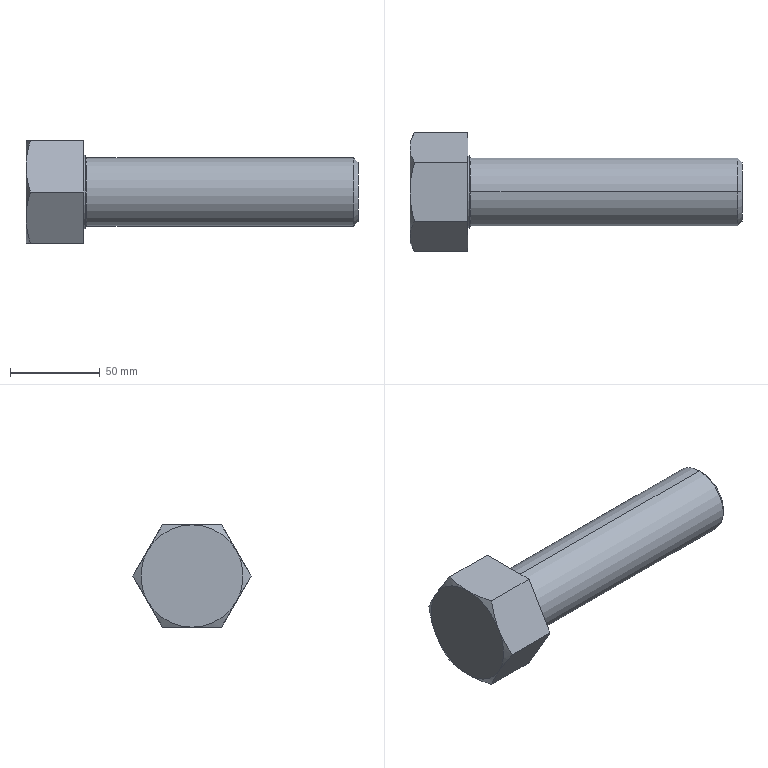Part | SolidWorks | features RevCut 4, Chamfer 1, Extrusion 1, Fillet 1, LPattern 1, Revolution 1 | 1 solid | 24 faces | box 185.42 x 65.991 x 57.15 mm | volume 265435 mm3 | plane 10 | cone 8 | cylinder 4 | torus 2 | commonest cylinder face diameters 38.1 x2 41 x2
STEP:
#1=CARTESIAN_POINT('',(34.02,0.,19.05));
#2=VERTEX_POINT('',#1);
#3=CARTESIAN_POINT('',(34.02,0.,-19.05));
#4=VERTEX_POINT('',#3);
#5=CARTESIAN_POINT('',(34.02,0.,0.));
#6=DIRECTION('',(1.,0.,0.));
#7=DIRECTION('',(0.,0.,-1.));
#8=AXIS2_PLACEMENT_3D('',#5,#6,#7);
#9=CIRCLE('',#8,19.05);
#10=EDGE_CURVE('',#2,#4,#9,.T.);
#11=ORIENTED_EDGE('',*,*,#10,.F.);
#12=CARTESIAN_POINT('',(33.02,0.,20.05));
#13=VERTEX_POINT('',#12);
#14=CARTESIAN_POINT('',(34.02,0.,20.05));
#15=DIRECTION('',(0.,1.,0.));
#16=DIRECTION('',(0.,0.,1.));
#17=AXIS2_PLACEMENT_3D('',#14,#15,#16);
#18=CIRCLE('',#17,1.);
#19=EDGE_CURVE('',#2,#13,#18,.T.);
#20=ORIENTED_EDGE('',*,*,#19,.T.);
#21=CARTESIAN_POINT('',(33.02,0.,-20.05));
#22=VERTEX_POINT('',#21);
#23=CARTESIAN_POINT('',(33.02,0.,0.));
#24=DIRECTION('',(-1.,0.,0.));
#25=DIRECTION('',(0.,0.,-1.));
#26=AXIS2_PLACEMENT_3D('',#23,#24,#25);
#27=CIRCLE('',#26,20.05);
#28=EDGE_CURVE('',#22,#13,#27,.T.);
#29=ORIENTED_EDGE('',*,*,#28,.F.);
#30=CARTESIAN_POINT('',(34.02,0.,-20.05));
#31=DIRECTION('',(0.,-1.,0.));
#32=DIRECTION('',(0.,0.,-1.));
#33=AXIS2_PLACEMENT_3D('',#30,#31,#32);
#34=CIRCLE('',#33,1.);
#35=EDGE_CURVE('',#4,#22,#34,.T.);
#36=ORIENTED_EDGE('',*,*,#35,.F.);
#37=EDGE_LOOP('',(#11,#20,#29,#36));
#38=FACE_OUTER_BOUND('',#37,.T.);
#39=CARTESIAN_POINT('',(34.02,0.,0.));
#40=DIRECTION('',(1.,0.,0.));
#41=DIRECTION('',(0.,0.,-1.));
#42=AXIS2_PLACEMENT_3D('',#39,#40,#41);
#43=TOROIDAL_SURFACE('',#42,20.05,1.);
#44=ADVANCED_FACE('',(#38),#43,.F.);
#45=CARTESIAN_POINT('',(185.42,0.,-16.65));
#46=VERTEX_POINT('',#45);
#47=CARTESIAN_POINT('',(185.42,0.,16.65));
#48=VERTEX_POINT('',#47);
#49=CARTESIAN_POINT('',(185.42,0.,0.));
#50=DIRECTION('',(1.,0.,0.));
#51=DIRECTION('',(0.,0.,1.));
#52=AXIS2_PLACEMENT_3D('',#49,#50,#51);
#53=CIRCLE('',#52,16.65);
#54=EDGE_CURVE('',#46,#48,#53,.T.);
#55=ORIENTED_EDGE('',*,*,#54,.F.);
#56=CARTESIAN_POINT('',(183.02,0.,-19.05));
#57=VERTEX_POINT('',#56);
#58=CARTESIAN_POINT('',(183.02,0.,-19.05));
#59=DIRECTION('',(-0.7071,0.,-0.7071));
#60=VECTOR('',#59,1000.);
#61=LINE('',#58,#60);
#62=EDGE_CURVE('',#46,#57,#61,.T.);
#63=ORIENTED_EDGE('',*,*,#62,.T.);
#64=CARTESIAN_POINT('',(183.02,0.,19.05));
#65=VERTEX_POINT('',#64);
#66=CARTESIAN_POINT('',(183.02,0.,0.));
#67=DIRECTION('',(-1.,0.,0.));
#68=DIRECTION('',(0.,0.,1.));
#69=AXIS2_PLACEMENT_3D('',#66,#67,#68);
#70=CIRCLE('',#69,19.05);
#71=EDGE_CURVE('',#65,#57,#70,.T.);
#72=ORIENTED_EDGE('',*,*,#71,.F.);
#73=CARTESIAN_POINT('',(183.02,0.,19.05));
#74=DIRECTION('',(-0.7071,0.,0.7071));
#75=VECTOR('',#74,1000.);
#76=LINE('',#73,#75);
#77=EDGE_CURVE('',#48,#65,#76,.T.);
#78=ORIENTED_EDGE('',*,*,#77,.F.);
#79=EDGE_LOOP('',(#55,#63,#72,#78));
#80=FACE_OUTER_BOUND('',#79,.T.);
#81=CARTESIAN_POINT('',(183.02,0.,0.));
#82=DIRECTION('',(-1.,0.,0.));
#83=DIRECTION('',(0.,0.,1.));
#84=AXIS2_PLACEMENT_3D('',#81,#82,#83);
#85=CONICAL_SURFACE('',#84,19.05,0.7854);
#86=ADVANCED_FACE('',(#80),#85,.T.);
#87=ORIENTED_EDGE('',*,*,#71,.T.);
#88=CARTESIAN_POINT('',(0.,0.,-19.05));
#89=DIRECTION('',(-1.,0.,0.));
#90=VECTOR('',#89,1000.);
#91=LINE('',#88,#90);
#92=EDGE_CURVE('',#57,#4,#91,.T.);
#93=ORIENTED_EDGE('',*,*,#92,.T.);
#94=CARTESIAN_POINT('',(34.02,0.,0.));
#95=DIRECTION('',(1.,0.,0.));
#96=DIRECTION('',(0.,0.,-1.));
#97=AXIS2_PLACEMENT_3D('',#94,#95,#96);
#98=CIRCLE('',#97,19.05);
#99=EDGE_CURVE('',#4,#2,#98,.T.);
#100=ORIENTED_EDGE('',*,*,#99,.T.);
#101=CARTESIAN_POINT('',(0.,0.,19.05));
#102=DIRECTION('',(-1.,0.,0.));
#103=VECTOR('',#102,1000.);
#104=LINE('',#101,#103);
#105=EDGE_CURVE('',#65,#2,#104,.T.);
#106=ORIENTED_EDGE('',*,*,#105,.F.);
#107=EDGE_LOOP('',(#87,#93,#100,#106));
#108=FACE_OUTER_BOUND('',#107,.T.);
#109=CARTESIAN_POINT('',(0.,0.,0.));
#110=DIRECTION('',(-1.,0.,0.));
#111=DIRECTION('',(0.,0.,1.));
#112=AXIS2_PLACEMENT_3D('',#109,#110,#111);
#113=CYLINDRICAL_SURFACE('',#112,19.05);
#114=ADVANCED_FACE('',(#108),#113,.T.);
#115=CARTESIAN_POINT('',(33.02,0.,20.5));
#116=VERTEX_POINT('',#115);
#117=CARTESIAN_POINT('',(33.02,0.,-20.5));
#118=VERTEX_POINT('',#117);
#119=CARTESIAN_POINT('',(33.02,0.,0.));
#120=DIRECTION('',(-1.,0.,0.));
#121=DIRECTION('',(0.,0.,1.));
#122=AXIS2_PLACEMENT_3D('',#119,#120,#121);
#123=CIRCLE('',#122,20.5);
#124=EDGE_CURVE('',#116,#118,#123,.T.);
#125=ORIENTED_EDGE('',*,*,#124,.T.);
#126=CARTESIAN_POINT('',(32.22,0.,-20.5));
#127=VERTEX_POINT('',#126);
#128=CARTESIAN_POINT('',(0.,0.,-20.5));
#129=DIRECTION('',(-1.,0.,0.));
#130=VECTOR('',#129,1000.);
#131=LINE('',#128,#130);
#132=EDGE_CURVE('',#118,#127,#131,.T.);
#133=ORIENTED_EDGE('',*,*,#132,.T.);
#134=CARTESIAN_POINT('',(32.22,0.,20.5));
#135=VERTEX_POINT('',#134);
#136=CARTESIAN_POINT('',(32.22,0.,0.));
#137=DIRECTION('',(-1.,0.,0.));
#138=DIRECTION('',(0.,0.,1.));
#139=AXIS2_PLACEMENT_3D('',#136,#137,#138);
#140=CIRCLE('',#139,20.5);
#141=EDGE_CURVE('',#135,#127,#140,.T.);
#142=ORIENTED_EDGE('',*,*,#141,.F.);
#143=CARTESIAN_POINT('',(0.,0.,20.5));
#144=DIRECTION('',(-1.,0.,0.));
#145=VECTOR('',#144,1000.);
#146=LINE('',#143,#145);
#147=EDGE_CURVE('',#116,#135,#146,.T.);
#148=ORIENTED_EDGE('',*,*,#147,.F.);
#149=EDGE_LOOP('',(#125,#133,#142,#148));
#150=FACE_OUTER_BOUND('',#149,.T.);
#151=CARTESIAN_POINT('',(0.,0.,0.));
#152=DIRECTION('',(-1.,0.,0.));
#153=DIRECTION('',(0.,0.,1.));
#154=AXIS2_PLACEMENT_3D('',#151,#152,#153);
#155=CYLINDRICAL_SURFACE('',#154,20.5);
#156=ADVANCED_FACE('',(#150),#155,.T.);
#157=CARTESIAN_POINT('',(32.22,16.498,-28.575));
#158=VERTEX_POINT('',#157);
#159=CARTESIAN_POINT('',(32.22,32.996,0.));
#160=VERTEX_POINT('',#159);
#161=CARTESIAN_POINT('',(32.22,16.498,-28.575));
#162=DIRECTION('',(0.,0.5,0.866));
#163=VECTOR('',#162,1000.);
#164=LINE('',#161,#163);
#165=EDGE_CURVE('',#158,#160,#164,.T.);
#166=ORIENTED_EDGE('',*,*,#165,.F.);
#167=CARTESIAN_POINT('',(2.552,16.498,-28.575));
#168=VERTEX_POINT('',#167);
#169=CARTESIAN_POINT('',(33.02,16.498,-28.575));
#170=DIRECTION('',(-1.,0.,0.));
#171=VECTOR('',#170,1000.);
#172=LINE('',#169,#171);
#173=EDGE_CURVE('',#158,#168,#172,.T.);
#174=ORIENTED_EDGE('',*,*,#173,.T.);
#175=CARTESIAN_POINT('',(0.,24.747,-14.288));
#176=VERTEX_POINT('',#175);
#177=CARTESIAN_POINT('',(0.,24.747,-14.288));
#178=CARTESIAN_POINT('',(0.,24.397,-14.894));
#179=CARTESIAN_POINT('',(0.01497,24.045,-15.503));
#180=CARTESIAN_POINT('',(0.07434,23.345,-16.716));
#181=CARTESIAN_POINT('',(0.1187,22.996,-17.32));
#182=CARTESIAN_POINT('',(0.2938,21.952,-19.127));
#183=CARTESIAN_POINT('',(0.4667,21.261,-20.324));
#184=CARTESIAN_POINT('',(1.134,19.201,-23.893));
#185=CARTESIAN_POINT('',(1.775,17.844,-26.244));
#186=CARTESIAN_POINT('',(2.552,16.498,-28.575));
#187=B_SPLINE_CURVE_WITH_KNOTS('',3,(#177,#178,#179,#180,#181,#182,#183,#184,#185,#186),.UNSPECIFIED.,.F.,.F.,(4,2,2,2,4),(0.01669,0.01877,0.02085,0.02501,0.03332),.UNSPECIFIED.);
#188=EDGE_CURVE('',#176,#168,#187,.T.);
#189=ORIENTED_EDGE('',*,*,#188,.F.);
#190=CARTESIAN_POINT('',(2.552,32.996,0.));
#191=VERTEX_POINT('',#190);
#192=CARTESIAN_POINT('',(2.552,32.996,0.));
#193=CARTESIAN_POINT('',(1.773,31.646,-2.337));
#194=CARTESIAN_POINT('',(1.131,30.287,-4.692));
#195=CARTESIAN_POINT('',(0.2432,27.54,-9.449));
#196=CARTESIAN_POINT('',(0.,26.152,-11.853));
#197=CARTESIAN_POINT('',(0.,24.747,-14.288));
#198=B_SPLINE_CURVE_WITH_KNOTS('',3,(#192,#193,#194,#195,#196,#197),.UNSPECIFIED.,.F.,.F.,(4,2,4),(0.000000238,0.008347,0.01669),.UNSPECIFIED.);
#199=EDGE_CURVE('',#191,#176,#198,.T.);
#200=ORIENTED_EDGE('',*,*,#199,.F.);
#201=CARTESIAN_POINT('',(33.02,32.996,0.));
#202=DIRECTION('',(-1.,0.,0.));
#203=VECTOR('',#202,1000.);
#204=LINE('',#201,#203);
#205=EDGE_CURVE('',#160,#191,#204,.T.);
#206=ORIENTED_EDGE('',*,*,#205,.F.);
#207=EDGE_LOOP('',(#166,#174,#189,#200,#206));
#208=FACE_OUTER_BOUND('',#207,.T.);
#209=CARTESIAN_POINT('',(33.02,16.498,-28.575));
#210=DIRECTION('',(0.,-0.866,0.5));
#211=DIRECTION('',(0.,-0.5,-0.866));
#212=AXIS2_PLACEMENT_3D('',#209,#210,#211);
#213=PLANE('',#212);
#214=ADVANCED_FACE('',(#208),#213,.F.);
#215=CARTESIAN_POINT('',(32.22,16.498,28.575));
#216=VERTEX_POINT('',#215);
#217=CARTESIAN_POINT('',(32.22,32.996,0.));
#218=DIRECTION('',(0.,-0.5,0.866));
#219=VECTOR('',#218,1000.);
#220=LINE('',#217,#219);
#221=EDGE_CURVE('',#160,#216,#220,.T.);
#222=ORIENTED_EDGE('',*,*,#221,.F.);
#223=ORIENTED_EDGE('',*,*,#205,.T.);
#224=CARTESIAN_POINT('',(0.,24.747,14.288));
#225=VERTEX_POINT('',#224);
#226=CARTESIAN_POINT('',(0.,24.747,14.288));
#227=CARTESIAN_POINT('',(0.,25.097,13.681));
#228=CARTESIAN_POINT('',(0.01497,25.448,13.072));
#229=CARTESIAN_POINT('',(0.07434,26.149,11.859));
#230=CARTESIAN_POINT('',(0.1187,26.498,11.255));
#231=CARTESIAN_POINT('',(0.2938,27.541,9.448));
#232=CARTESIAN_POINT('',(0.4667,28.232,8.251));
#233=CARTESIAN_POINT('',(1.134,30.292,4.682));
#234=CARTESIAN_POINT('',(1.775,31.65,2.331));
#235=CARTESIAN_POINT('',(2.552,32.996,0.));
#236=B_SPLINE_CURVE_WITH_KNOTS('',3,(#226,#227,#228,#229,#230,#231,#232,#233,#234,#235),.UNSPECIFIED.,.F.,.F.,(4,2,2,2,4),(0.01669,0.01877,0.02085,0.02501,0.03332),.UNSPECIFIED.);
#237=EDGE_CURVE('',#225,#191,#236,.T.);
#238=ORIENTED_EDGE('',*,*,#237,.F.);
#239=CARTESIAN_POINT('',(2.552,16.498,28.575));
#240=VERTEX_POINT('',#239);
#241=CARTESIAN_POINT('',(2.552,16.498,28.575));
#242=CARTESIAN_POINT('',(1.773,17.847,26.238));
#243=CARTESIAN_POINT('',(1.131,19.206,23.883));
#244=CARTESIAN_POINT('',(0.2432,21.953,19.126));
#245=CARTESIAN_POINT('',(0.,23.341,16.722));
#246=CARTESIAN_POINT('',(0.,24.747,14.288));
#247=B_SPLINE_CURVE_WITH_KNOTS('',3,(#241,#242,#243,#244,#245,#246),.UNSPECIFIED.,.F.,.F.,(4,2,4),(0.000000238,0.008347,0.01669),.UNSPECIFIED.);
#248=EDGE_CURVE('',#240,#225,#247,.T.);
#249=ORIENTED_EDGE('',*,*,#248,.F.);
#250=CARTESIAN_POINT('',(33.02,16.498,28.575));
#251=DIRECTION('',(-1.,0.,0.));
#252=VECTOR('',#251,1000.);
#253=LINE('',#250,#252);
#254=EDGE_CURVE('',#216,#240,#253,.T.);
#255=ORIENTED_EDGE('',*,*,#254,.F.);
#256=EDGE_LOOP('',(#222,#223,#238,#249,#255));
#257=FACE_OUTER_BOUND('',#256,.T.);
#258=CARTESIAN_POINT('',(33.02,32.996,0.));
#259=DIRECTION('',(0.,-0.866,-0.5));
#260=DIRECTION('',(0.,0.5,-0.866));
#261=AXIS2_PLACEMENT_3D('',#258,#259,#260);
#262=PLANE('',#261);
#263=ADVANCED_FACE('',(#257),#262,.F.);
#264=CARTESIAN_POINT('',(32.22,-16.498,28.575));
#265=VERTEX_POINT('',#264);
#266=CARTESIAN_POINT('',(32.22,16.498,28.575));
#267=DIRECTION('',(0.,-1.,0.));
#268=VECTOR('',#267,1000.);
#269=LINE('',#266,#268);
#270=EDGE_CURVE('',#216,#265,#269,.T.);
#271=ORIENTED_EDGE('',*,*,#270,.F.);
#272=ORIENTED_EDGE('',*,*,#254,.T.);
#273=CARTESIAN_POINT('',(0.,0.,28.575));
#274=VERTEX_POINT('',#273);
#275=CARTESIAN_POINT('',(0.,0.,28.575));
#276=CARTESIAN_POINT('',(0.,1.395,28.575));
#277=CARTESIAN_POINT('',(0.05934,2.796,28.575));
#278=CARTESIAN_POINT('',(0.2953,5.606,28.575));
#279=CARTESIAN_POINT('',(0.4701,6.996,28.575));
#280=CARTESIAN_POINT('',(1.141,11.128,28.575));
#281=CARTESIAN_POINT('',(1.782,13.83,28.575));
#282=CARTESIAN_POINT('',(2.552,16.498,28.575));
#283=B_SPLINE_CURVE_WITH_KNOTS('',3,(#275,#276,#277,#278,#279,#280,#281,#282),.UNSPECIFIED.,.F.,.F.,(4,2,2,4),(0.04657,0.05075,0.05493,0.06328),.UNSPECIFIED.);
#284=EDGE_CURVE('',#274,#240,#283,.T.);
#285=ORIENTED_EDGE('',*,*,#284,.F.);
#286=CARTESIAN_POINT('',(2.552,-16.498,28.575));
#287=VERTEX_POINT('',#286);
#288=CARTESIAN_POINT('',(2.552,-16.498,28.575));
#289=CARTESIAN_POINT('',(2.165,-15.156,28.575));
#290=CARTESIAN_POINT('',(1.809,-13.8,28.575));
#291=CARTESIAN_POINT('',(1.178,-11.061,28.575));
#292=CARTESIAN_POINT('',(0.9058,-9.689,28.575));
#293=CARTESIAN_POINT('',(0.2398,-5.559,28.575));
#294=CARTESIAN_POINT('',(0.,-2.789,28.575));
#295=CARTESIAN_POINT('',(0.,0.,28.575));
#296=B_SPLINE_CURVE_WITH_KNOTS('',3,(#288,#289,#290,#291,#292,#293,#294,#295),.UNSPECIFIED.,.F.,.F.,(4,2,2,4),(0.02988,0.03405,0.03823,0.04657),.UNSPECIFIED.);
#297=EDGE_CURVE('',#287,#274,#296,.T.);
#298=ORIENTED_EDGE('',*,*,#297,.F.);
#299=CARTESIAN_POINT('',(33.02,-16.498,28.575));
#300=DIRECTION('',(-1.,0.,0.));
#301=VECTOR('',#300,1000.);
#302=LINE('',#299,#301);
#303=EDGE_CURVE('',#265,#287,#302,.T.);
#304=ORIENTED_EDGE('',*,*,#303,.F.);
#305=EDGE_LOOP('',(#271,#272,#285,#298,#304));
#306=FACE_OUTER_BOUND('',#305,.T.);
#307=CARTESIAN_POINT('',(33.02,16.498,28.575));
#308=DIRECTION('',(0.,0.,-1.));
#309=DIRECTION('',(0.,1.,0.));
#310=AXIS2_PLACEMENT_3D('',#307,#308,#309);
#311=PLANE('',#310);
#312=ADVANCED_FACE('',(#306),#311,.F.);
#313=CARTESIAN_POINT('',(32.22,-32.996,0.));
#314=VERTEX_POINT('',#313);
#315=CARTESIAN_POINT('',(32.22,-32.996,0.));
#316=DIRECTION('',(0.,-0.5,-0.866));
#317=VECTOR('',#316,1000.);
#318=LINE('',#315,#317);
#319=EDGE_CURVE('',#265,#314,#318,.T.);
#320=ORIENTED_EDGE('',*,*,#319,.F.);
#321=ORIENTED_EDGE('',*,*,#303,.T.);
#322=CARTESIAN_POINT('',(0.,-24.747,14.288));
#323=VERTEX_POINT('',#322);
#324=CARTESIAN_POINT('',(0.,-24.747,14.288));
#325=CARTESIAN_POINT('',(0.,-24.397,14.894));
#326=CARTESIAN_POINT('',(0.01497,-24.045,15.503));
#327=CARTESIAN_POINT('',(0.07434,-23.345,16.716));
#328=CARTESIAN_POINT('',(0.1187,-22.996,17.32));
#329=CARTESIAN_POINT('',(0.2938,-21.952,19.127));
#330=CARTESIAN_POINT('',(0.4667,-21.261,20.324));
#331=CARTESIAN_POINT('',(1.134,-19.201,23.893));
#332=CARTESIAN_POINT('',(1.775,-17.844,26.244));
#333=CARTESIAN_POINT('',(2.552,-16.498,28.575));
#334=B_SPLINE_CURVE_WITH_KNOTS('',3,(#324,#325,#326,#327,#328,#329,#330,#331,#332,#333),.UNSPECIFIED.,.F.,.F.,(4,2,2,2,4),(0.01669,0.01877,0.02085,0.02501,0.03332),.UNSPECIFIED.);
#335=EDGE_CURVE('',#323,#287,#334,.T.);
#336=ORIENTED_EDGE('',*,*,#335,.F.);
#337=CARTESIAN_POINT('',(2.552,-32.996,0.));
#338=VERTEX_POINT('',#337);
#339=CARTESIAN_POINT('',(2.552,-32.996,0.));
#340=CARTESIAN_POINT('',(1.773,-31.646,2.337));
#341=CARTESIAN_POINT('',(1.131,-30.287,4.692));
#342=CARTESIAN_POINT('',(0.2432,-27.54,9.449));
#343=CARTESIAN_POINT('',(0.,-26.152,11.853));
#344=CARTESIAN_POINT('',(0.,-24.747,14.288));
#345=B_SPLINE_CURVE_WITH_KNOTS('',3,(#339,#340,#341,#342,#343,#344),.UNSPECIFIED.,.F.,.F.,(4,2,4),(0.000000238,0.008347,0.01669),.UNSPECIFIED.);
#346=EDGE_CURVE('',#338,#323,#345,.T.);
#347=ORIENTED_EDGE('',*,*,#346,.F.);
#348=CARTESIAN_POINT('',(33.02,-32.996,0.));
#349=DIRECTION('',(-1.,0.,0.));
#350=VECTOR('',#349,1000.);
#351=LINE('',#348,#350);
#352=EDGE_CURVE('',#314,#338,#351,.T.);
#353=ORIENTED_EDGE('',*,*,#352,.F.);
#354=EDGE_LOOP('',(#320,#321,#336,#347,#353));
#355=FACE_OUTER_BOUND('',#354,.T.);
#356=CARTESIAN_POINT('',(33.02,-32.996,0.));
#357=DIRECTION('',(0.,0.866,-0.5));
#358=DIRECTION('',(0.,0.5,0.866));
#359=AXIS2_PLACEMENT_3D('',#356,#357,#358);
#360=PLANE('',#359);
#361=ADVANCED_FACE('',(#355),#360,.F.);
#362=CARTESIAN_POINT('',(32.22,-16.498,-28.575));
#363=VERTEX_POINT('',#362);
#364=CARTESIAN_POINT('',(32.22,-16.498,-28.575));
#365=DIRECTION('',(0.,0.5,-0.866));
#366=VECTOR('',#365,1000.);
#367=LINE('',#364,#366);
#368=EDGE_CURVE('',#314,#363,#367,.T.);
#369=ORIENTED_EDGE('',*,*,#368,.F.);
#370=ORIENTED_EDGE('',*,*,#352,.T.);
#371=CARTESIAN_POINT('',(0.,-24.747,-14.288));
#372=VERTEX_POINT('',#371);
#373=CARTESIAN_POINT('',(0.,-24.747,-14.288));
#374=CARTESIAN_POINT('',(0.,-25.097,-13.681));
#375=CARTESIAN_POINT('',(0.01497,-25.448,-13.072));
#376=CARTESIAN_POINT('',(0.07434,-26.149,-11.859));
#377=CARTESIAN_POINT('',(0.1187,-26.498,-11.255));
#378=CARTESIAN_POINT('',(0.2938,-27.541,-9.448));
#379=CARTESIAN_POINT('',(0.4667,-28.232,-8.251));
#380=CARTESIAN_POINT('',(1.134,-30.292,-4.682));
#381=CARTESIAN_POINT('',(1.775,-31.65,-2.331));
#382=CARTESIAN_POINT('',(2.552,-32.996,0.));
#383=B_SPLINE_CURVE_WITH_KNOTS('',3,(#373,#374,#375,#376,#377,#378,#379,#380,#381,#382),.UNSPECIFIED.,.F.,.F.,(4,2,2,2,4),(0.01669,0.01877,0.02085,0.02501,0.03332),.UNSPECIFIED.);
#384=EDGE_CURVE('',#372,#338,#383,.T.);
#385=ORIENTED_EDGE('',*,*,#384,.F.);
#386=CARTESIAN_POINT('',(2.552,-16.498,-28.575));
#387=VERTEX_POINT('',#386);
#388=CARTESIAN_POINT('',(2.552,-16.498,-28.575));
#389=CARTESIAN_POINT('',(1.773,-17.847,-26.238));
#390=CARTESIAN_POINT('',(1.131,-19.206,-23.883));
#391=CARTESIAN_POINT('',(0.2432,-21.953,-19.126));
#392=CARTESIAN_POINT('',(0.,-23.341,-16.722));
#393=CARTESIAN_POINT('',(0.,-24.747,-14.288));
#394=B_SPLINE_CURVE_WITH_KNOTS('',3,(#388,#389,#390,#391,#392,#393),.UNSPECIFIED.,.F.,.F.,(4,2,4),(0.000000238,0.008347,0.01669),.UNSPECIFIED.);
#395=EDGE_CURVE('',#387,#372,#394,.T.);
#396=ORIENTED_EDGE('',*,*,#395,.F.);
#397=CARTESIAN_POINT('',(33.02,-16.498,-28.575));
#398=DIRECTION('',(-1.,0.,0.));
#399=VECTOR('',#398,1000.);
#400=LINE('',#397,#399);
#401=EDGE_CURVE('',#363,#387,#400,.T.);
#402=ORIENTED_EDGE('',*,*,#401,.F.);
#403=EDGE_LOOP('',(#369,#370,#385,#396,#402));
#404=FACE_OUTER_BOUND('',#403,.T.);
#405=CARTESIAN_POINT('',(33.02,-16.498,-28.575));
#406=DIRECTION('',(0.,0.866,0.5));
#407=DIRECTION('',(0.,-0.5,0.866));
#408=AXIS2_PLACEMENT_3D('',#405,#406,#407);
#409=PLANE('',#408);
#410=ADVANCED_FACE('',(#404),#409,.F.);
#411=CARTESIAN_POINT('',(32.22,16.498,-28.575));
#412=DIRECTION('',(0.,1.,0.));
#413=VECTOR('',#412,1000.);
#414=LINE('',#411,#413);
#415=EDGE_CURVE('',#363,#158,#414,.T.);
#416=ORIENTED_EDGE('',*,*,#415,.F.);
#417=ORIENTED_EDGE('',*,*,#401,.T.);
#418=CARTESIAN_POINT('',(0.,0.,-28.575));
#419=VERTEX_POINT('',#418);
#420=CARTESIAN_POINT('',(0.,0.,-28.575));
#421=CARTESIAN_POINT('',(0.,-2.789,-28.575));
#422=CARTESIAN_POINT('',(0.2398,-5.559,-28.575));
#423=CARTESIAN_POINT('',(0.9058,-9.689,-28.575));
#424=CARTESIAN_POINT('',(1.178,-11.061,-28.575));
#425=CARTESIAN_POINT('',(1.809,-13.8,-28.575));
#426=CARTESIAN_POINT('',(2.165,-15.156,-28.575));
#427=CARTESIAN_POINT('',(2.552,-16.498,-28.575));
#428=B_SPLINE_CURVE_WITH_KNOTS('',3,(#420,#421,#422,#423,#424,#425,#426,#427),.UNSPECIFIED.,.F.,.F.,(4,2,2,4),(0.09019,0.09855,0.1027,0.1069),.UNSPECIFIED.);
#429=EDGE_CURVE('',#419,#387,#428,.T.);
#430=ORIENTED_EDGE('',*,*,#429,.F.);
#431=CARTESIAN_POINT('',(2.552,16.498,-28.575));
#432=CARTESIAN_POINT('',(1.782,13.83,-28.575));
#433=CARTESIAN_POINT('',(1.141,11.128,-28.575));
#434=CARTESIAN_POINT('',(0.4701,6.996,-28.575));
#435=CARTESIAN_POINT('',(0.2953,5.606,-28.575));
#436=CARTESIAN_POINT('',(0.05934,2.796,-28.575));
#437=CARTESIAN_POINT('',(0.,1.395,-28.575));
#438=CARTESIAN_POINT('',(0.,0.,-28.575));
#439=B_SPLINE_CURVE_WITH_KNOTS('',3,(#431,#432,#433,#434,#435,#436,#437,#438),.UNSPECIFIED.,.F.,.F.,(4,2,2,4),(0.07347,0.08183,0.08601,0.09019),.UNSPECIFIED.);
#440=EDGE_CURVE('',#168,#419,#439,.T.);
#441=ORIENTED_EDGE('',*,*,#440,.F.);
#442=ORIENTED_EDGE('',*,*,#173,.F.);
#443=EDGE_LOOP('',(#416,#417,#430,#441,#442));
#444=FACE_OUTER_BOUND('',#443,.T.);
#445=CARTESIAN_POINT('',(33.02,16.498,-28.575));
#446=DIRECTION('',(0.,0.,1.));
#447=DIRECTION('',(0.,-1.,0.));
#448=AXIS2_PLACEMENT_3D('',#445,#446,#447);
#449=PLANE('',#448);
#450=ADVANCED_FACE('',(#444),#449,.F.);
#451=ORIENTED_EDGE('',*,*,#395,.T.);
#452=CARTESIAN_POINT('',(0.,0.,0.));
#453=DIRECTION('',(1.,0.,0.));
#454=DIRECTION('',(0.,0.,-1.));
#455=AXIS2_PLACEMENT_3D('',#452,#453,#454);
#456=CIRCLE('',#455,28.575);
#457=EDGE_CURVE('',#372,#419,#456,.T.);
#458=ORIENTED_EDGE('',*,*,#457,.T.);
#459=ORIENTED_EDGE('',*,*,#429,.T.);
#460=EDGE_LOOP('',(#451,#458,#459));
#461=FACE_OUTER_BOUND('',#460,.T.);
#462=CARTESIAN_POINT('',(0.,0.,0.));
#463=DIRECTION('',(1.,0.,0.));
#464=DIRECTION('',(0.,0.,-1.));
#465=AXIS2_PLACEMENT_3D('',#462,#463,#464);
#466=CONICAL_SURFACE('',#465,28.575,1.047);
#467=ADVANCED_FACE('',(#461),#466,.T.);
#468=ORIENTED_EDGE('',*,*,#346,.T.);
#469=CARTESIAN_POINT('',(0.,0.,0.));
#470=DIRECTION('',(1.,0.,0.));
#471=DIRECTION('',(0.,0.,-1.));
#472=AXIS2_PLACEMENT_3D('',#469,#470,#471);
#473=CIRCLE('',#472,28.575);
#474=EDGE_CURVE('',#323,#372,#473,.T.);
#475=ORIENTED_EDGE('',*,*,#474,.T.);
#476=ORIENTED_EDGE('',*,*,#384,.T.);
#477=EDGE_LOOP('',(#468,#475,#476));
#478=FACE_OUTER_BOUND('',#477,.T.);
#479=CARTESIAN_POINT('',(0.,0.,0.));
#480=DIRECTION('',(1.,0.,0.));
#481=DIRECTION('',(0.,0.,-1.));
#482=AXIS2_PLACEMENT_3D('',#479,#480,#481);
#483=CONICAL_SURFACE('',#482,28.575,1.047);
#484=ADVANCED_FACE('',(#478),#483,.T.);
#485=ORIENTED_EDGE('',*,*,#297,.T.);
#486=CARTESIAN_POINT('',(0.,0.,0.));
#487=DIRECTION('',(1.,0.,0.));
#488=DIRECTION('',(0.,0.,-1.));
#489=AXIS2_PLACEMENT_3D('',#486,#487,#488);
#490=CIRCLE('',#489,28.575);
#491=EDGE_CURVE('',#274,#323,#490,.T.);
#492=ORIENTED_EDGE('',*,*,#491,.T.);
#493=ORIENTED_EDGE('',*,*,#335,.T.);
#494=EDGE_LOOP('',(#485,#492,#493));
#495=FACE_OUTER_BOUND('',#494,.T.);
#496=CARTESIAN_POINT('',(0.,0.,0.));
#497=DIRECTION('',(1.,0.,0.));
#498=DIRECTION('',(0.,0.,-1.));
#499=AXIS2_PLACEMENT_3D('',#496,#497,#498);
#500=CONICAL_SURFACE('',#499,28.575,1.047);
#501=ADVANCED_FACE('',(#495),#500,.T.);
#502=ORIENTED_EDGE('',*,*,#284,.T.);
#503=ORIENTED_EDGE('',*,*,#248,.T.);
#504=CARTESIAN_POINT('',(0.,0.,0.));
#505=DIRECTION('',(-1.,0.,0.));
#506=DIRECTION('',(0.,0.,1.));
#507=AXIS2_PLACEMENT_3D('',#504,#505,#506);
#508=CIRCLE('',#507,28.575);
#509=EDGE_CURVE('',#274,#225,#508,.T.);
#510=ORIENTED_EDGE('',*,*,#509,.F.);
#511=EDGE_LOOP('',(#502,#503,#510));
#512=FACE_OUTER_BOUND('',#511,.T.);
#513=CARTESIAN_POINT('',(0.,0.,0.));
#514=DIRECTION('',(1.,0.,0.));
#515=DIRECTION('',(0.,0.,-1.));
#516=AXIS2_PLACEMENT_3D('',#513,#514,#515);
#517=CONICAL_SURFACE('',#516,28.575,1.047);
#518=ADVANCED_FACE('',(#512),#517,.T.);
#519=ORIENTED_EDGE('',*,*,#237,.T.);
#520=ORIENTED_EDGE('',*,*,#199,.T.);
#521=CARTESIAN_POINT('',(0.,0.,0.));
#522=DIRECTION('',(1.,0.,0.));
#523=DIRECTION('',(0.,0.,-1.));
#524=AXIS2_PLACEMENT_3D('',#521,#522,#523);
#525=CIRCLE('',#524,28.575);
#526=EDGE_CURVE('',#176,#225,#525,.T.);
#527=ORIENTED_EDGE('',*,*,#526,.T.);
#528=EDGE_LOOP('',(#519,#520,#527));
#529=FACE_OUTER_BOUND('',#528,.T.);
#530=CARTESIAN_POINT('',(0.,0.,0.));
#531=DIRECTION('',(1.,0.,0.));
#532=DIRECTION('',(0.,0.,-1.));
#533=AXIS2_PLACEMENT_3D('',#530,#531,#532);
#534=CONICAL_SURFACE('',#533,28.575,1.047);
#535=ADVANCED_FACE('',(#529),#534,.T.);
#536=ORIENTED_EDGE('',*,*,#188,.T.);
#537=ORIENTED_EDGE('',*,*,#440,.T.);
#538=CARTESIAN_POINT('',(0.,0.,0.));
#539=DIRECTION('',(1.,0.,0.));
#540=DIRECTION('',(0.,0.,-1.));
#541=AXIS2_PLACEMENT_3D('',#538,#539,#540);
#542=CIRCLE('',#541,28.575);
#543=EDGE_CURVE('',#419,#176,#542,.T.);
#544=ORIENTED_EDGE('',*,*,#543,.T.);
#545=EDGE_LOOP('',(#536,#537,#544));
#546=FACE_OUTER_BOUND('',#545,.T.);
#547=CARTESIAN_POINT('',(0.,0.,0.));
#548=DIRECTION('',(1.,0.,0.));
#549=DIRECTION('',(0.,0.,-1.));
#550=AXIS2_PLACEMENT_3D('',#547,#548,#549);
#551=CONICAL_SURFACE('',#550,28.575,1.047);
#552=ADVANCED_FACE('',(#546),#551,.T.);
#553=ORIENTED_EDGE('',*,*,#543,.F.);
#554=ORIENTED_EDGE('',*,*,#457,.F.);
#555=ORIENTED_EDGE('',*,*,#474,.F.);
#556=ORIENTED_EDGE('',*,*,#491,.F.);
#557=ORIENTED_EDGE('',*,*,#509,.T.);
#558=ORIENTED_EDGE('',*,*,#526,.F.);
#559=EDGE_LOOP('',(#553,#554,#555,#556,#557,#558));
#560=FACE_OUTER_BOUND('',#559,.T.);
#561=CARTESIAN_POINT('',(0.,0.,-57.15));
#562=DIRECTION('',(1.,0.,0.));
#563=DIRECTION('',(0.,0.,-1.));
#564=AXIS2_PLACEMENT_3D('',#561,#562,#563);
#565=PLANE('',#564);
#566=ADVANCED_FACE('',(#560),#565,.F.);
#567=ORIENTED_EDGE('',*,*,#141,.T.);
#568=CARTESIAN_POINT('',(32.22,0.,0.));
#569=DIRECTION('',(-1.,0.,0.));
#570=DIRECTION('',(0.,0.,1.));
#571=AXIS2_PLACEMENT_3D('',#568,#569,#570);
#572=CIRCLE('',#571,20.5);
#573=EDGE_CURVE('',#127,#135,#572,.T.);
#574=ORIENTED_EDGE('',*,*,#573,.T.);
#575=EDGE_LOOP('',(#567,#574));
#576=FACE_BOUND('',#575,.T.);
#577=ORIENTED_EDGE('',*,*,#165,.T.);
#578=ORIENTED_EDGE('',*,*,#221,.T.);
#579=ORIENTED_EDGE('',*,*,#270,.T.);
#580=ORIENTED_EDGE('',*,*,#319,.T.);
#581=ORIENTED_EDGE('',*,*,#368,.T.);
#582=ORIENTED_EDGE('',*,*,#415,.T.);
#583=EDGE_LOOP('',(#577,#578,#579,#580,#581,#582));
#584=FACE_OUTER_BOUND('',#583,.T.);
#585=CARTESIAN_POINT('',(32.22,20.5,0.));
#586=DIRECTION('',(1.,0.,0.));
#587=DIRECTION('',(0.,0.,-1.));
#588=AXIS2_PLACEMENT_3D('',#585,#586,#587);
#589=PLANE('',#588);
#590=ADVANCED_FACE('',(#576,#584),#589,.T.);
#591=ORIENTED_EDGE('',*,*,#132,.F.);
#592=CARTESIAN_POINT('',(33.02,0.,0.));
#593=DIRECTION('',(-1.,0.,0.));
#594=DIRECTION('',(0.,0.,1.));
#595=AXIS2_PLACEMENT_3D('',#592,#593,#594);
#596=CIRCLE('',#595,20.5);
#597=EDGE_CURVE('',#118,#116,#596,.T.);
#598=ORIENTED_EDGE('',*,*,#597,.T.);
#599=ORIENTED_EDGE('',*,*,#147,.T.);
#600=ORIENTED_EDGE('',*,*,#573,.F.);
#601=EDGE_LOOP('',(#591,#598,#599,#600));
#602=FACE_OUTER_BOUND('',#601,.T.);
#603=CARTESIAN_POINT('',(0.,0.,0.));
#604=DIRECTION('',(-1.,0.,0.));
#605=DIRECTION('',(0.,0.,1.));
#606=AXIS2_PLACEMENT_3D('',#603,#604,#605);
#607=CYLINDRICAL_SURFACE('',#606,20.5);
#608=ADVANCED_FACE('',(#602),#607,.T.);
#609=CARTESIAN_POINT('',(185.42,0.,0.));
#610=DIRECTION('',(1.,0.,0.));
#611=DIRECTION('',(0.,0.,1.));
#612=AXIS2_PLACEMENT_3D('',#609,#610,#611);
#613=CIRCLE('',#612,16.65);
#614=EDGE_CURVE('',#48,#46,#613,.T.);
#615=ORIENTED_EDGE('',*,*,#614,.T.);
#616=ORIENTED_EDGE('',*,*,#54,.T.);
#617=EDGE_LOOP('',(#615,#616));
#618=FACE_OUTER_BOUND('',#617,.T.);
#619=CARTESIAN_POINT('',(185.42,0.,0.));
#620=DIRECTION('',(-1.,0.,0.));
#621=DIRECTION('',(0.,0.,1.));
#622=AXIS2_PLACEMENT_3D('',#619,#620,#621);
#623=PLANE('',#622);
#624=ADVANCED_FACE('',(#618),#623,.F.);
#625=ORIENTED_EDGE('',*,*,#92,.F.);
#626=CARTESIAN_POINT('',(183.02,0.,0.));
#627=DIRECTION('',(-1.,0.,0.));
#628=DIRECTION('',(0.,0.,1.));
#629=AXIS2_PLACEMENT_3D('',#626,#627,#628);
#630=CIRCLE('',#629,19.05);
#631=EDGE_CURVE('',#57,#65,#630,.T.);
#632=ORIENTED_EDGE('',*,*,#631,.T.);
#633=ORIENTED_EDGE('',*,*,#105,.T.);
#634=ORIENTED_EDGE('',*,*,#10,.T.);
#635=EDGE_LOOP('',(#625,#632,#633,#634));
#636=FACE_OUTER_BOUND('',#635,.T.);
#637=CARTESIAN_POINT('',(0.,0.,0.));
#638=DIRECTION('',(-1.,0.,0.));
#639=DIRECTION('',(0.,0.,1.));
#640=AXIS2_PLACEMENT_3D('',#637,#638,#639);
#641=CYLINDRICAL_SURFACE('',#640,19.05);
#642=ADVANCED_FACE('',(#636),#641,.T.);
#643=ORIENTED_EDGE('',*,*,#28,.T.);
#644=CARTESIAN_POINT('',(33.02,0.,0.));
#645=DIRECTION('',(-1.,0.,0.));
#646=DIRECTION('',(0.,0.,-1.));
#647=AXIS2_PLACEMENT_3D('',#644,#645,#646);
#648=CIRCLE('',#647,20.05);
#649=EDGE_CURVE('',#13,#22,#648,.T.);
#650=ORIENTED_EDGE('',*,*,#649,.T.);
#651=EDGE_LOOP('',(#643,#650));
#652=FACE_BOUND('',#651,.T.);
#653=ORIENTED_EDGE('',*,*,#124,.F.);
#654=ORIENTED_EDGE('',*,*,#597,.F.);
#655=EDGE_LOOP('',(#653,#654));
#656=FACE_OUTER_BOUND('',#655,.T.);
#657=CARTESIAN_POINT('',(33.02,0.,-57.15));
#658=DIRECTION('',(1.,0.,0.));
#659=DIRECTION('',(0.,0.,-1.));
#660=AXIS2_PLACEMENT_3D('',#657,#658,#659);
#661=PLANE('',#660);
#662=ADVANCED_FACE('',(#652,#656),#661,.T.);
#663=ORIENTED_EDGE('',*,*,#62,.F.);
#664=ORIENTED_EDGE('',*,*,#614,.F.);
#665=ORIENTED_EDGE('',*,*,#77,.T.);
#666=ORIENTED_EDGE('',*,*,#631,.F.);
#667=EDGE_LOOP('',(#663,#664,#665,#666));
#668=FACE_OUTER_BOUND('',#667,.T.);
#669=CARTESIAN_POINT('',(183.02,0.,0.));
#670=DIRECTION('',(-1.,0.,0.));
#671=DIRECTION('',(0.,0.,1.));
#672=AXIS2_PLACEMENT_3D('',#669,#670,#671);
#673=CONICAL_SURFACE('',#672,19.05,0.7854);
#674=ADVANCED_FACE('',(#668),#673,.T.);
#675=ORIENTED_EDGE('',*,*,#19,.F.);
#676=ORIENTED_EDGE('',*,*,#99,.F.);
#677=ORIENTED_EDGE('',*,*,#35,.T.);
#678=ORIENTED_EDGE('',*,*,#649,.F.);
#679=EDGE_LOOP('',(#675,#676,#677,#678));
#680=FACE_OUTER_BOUND('',#679,.T.);
#681=CARTESIAN_POINT('',(34.02,0.,0.));
#682=DIRECTION('',(1.,0.,0.));
#683=DIRECTION('',(0.,0.,-1.));
#684=AXIS2_PLACEMENT_3D('',#681,#682,#683);
#685=TOROIDAL_SURFACE('',#684,20.05,1.);
#686=ADVANCED_FACE('',(#680),#685,.F.);
#687=CLOSED_SHELL('',(#44,#86,#114,#156,#214,#263,#312,#361,#410,#450,#467,#484,#501,#518,#535,#552,#566,#590,#608,#624,#642,#662,#674,#686));
#688=MANIFOLD_SOLID_BREP('',#687);
#689=CARTESIAN_POINT('',(0.,0.,0.));
#690=DIRECTION('',(0.,0.,1.));
#691=DIRECTION('',(1.,0.,0.));
#692=AXIS2_PLACEMENT_3D('',#689,#690,#691);
#693=(LENGTH_UNIT()NAMED_UNIT(*)SI_UNIT(.MILLI.,.METRE.));
#694=UNCERTAINTY_MEASURE_WITH_UNIT(LENGTH_MEASURE(0.00001),#693,'','');
#695=(NAMED_UNIT(*)PLANE_ANGLE_UNIT()SI_UNIT($,.RADIAN.));
#696=(NAMED_UNIT(*)SI_UNIT($,.STERADIAN.)SOLID_ANGLE_UNIT());
#697=(GEOMETRIC_REPRESENTATION_CONTEXT(3)GLOBAL_UNCERTAINTY_ASSIGNED_CONTEXT((#694))GLOBAL_UNIT_ASSIGNED_CONTEXT((#693,#695,#696))REPRESENTATION_CONTEXT('',''));
#698=ADVANCED_BREP_SHAPE_REPRESENTATION('',(#688,#692),#697);